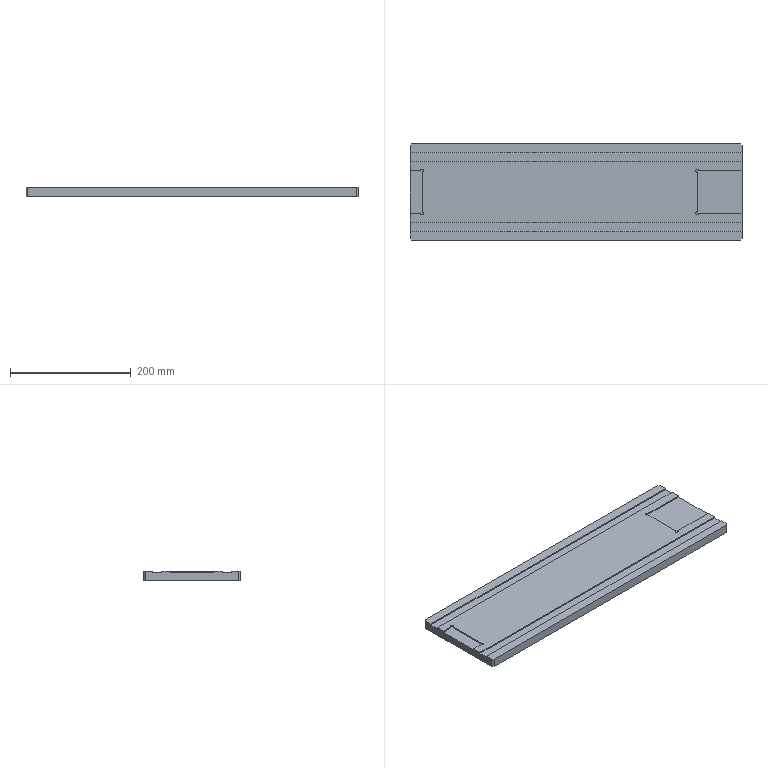Part | STEP file | 001-008-Traverse module base plate | 1 solid | 32 faces | box 549.5 x 160 x 15 mm | volume 1271693 mm3 | plane 26 | cylinder 6 | commonest cylinder face diameters 5 x6